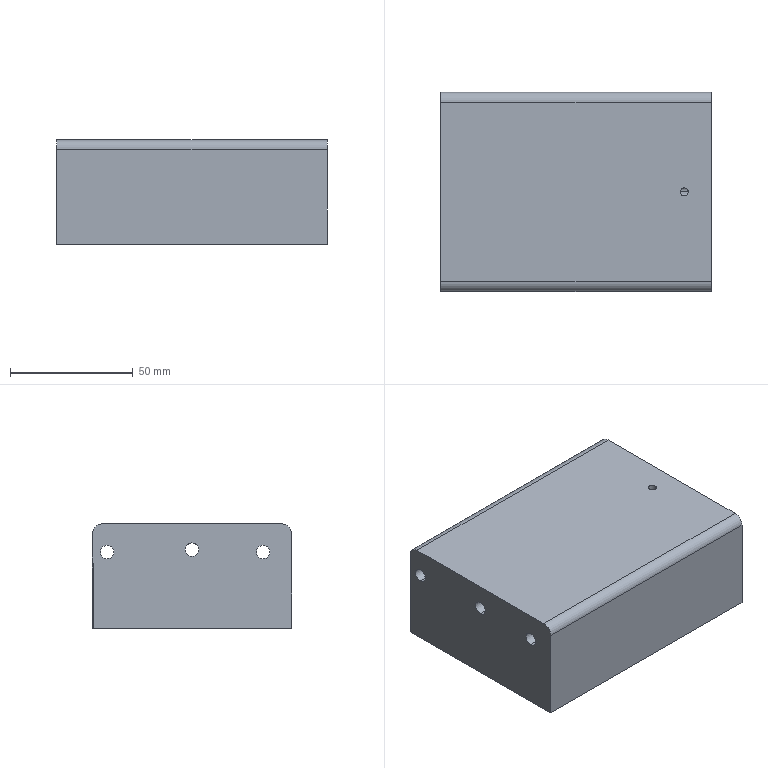Part | STEP file | FFH80-GY-002A^FFH85-B3 -02_three-axis module | 1 solid | 44 faces | box 110 x 81 x 42.5 mm | volume 368601 mm3 | cylinder 25 | plane 13 | cone 6 | commonest cylinder face diameters 5.5 x6 9 x6 4.2 x4 2.5 x2 3 x2 3.3 x2
STEP:
#1=CARTESIAN_POINT('',(102.,18.4,-2.25));
#2=VERTEX_POINT('',#1);
#3=CARTESIAN_POINT('',(102.,22.6,-2.25));
#4=VERTEX_POINT('',#3);
#5=CARTESIAN_POINT('',(102.,20.5,-2.25));
#6=DIRECTION('',(0.,0.,-1.));
#7=DIRECTION('',(0.,1.,0.));
#8=AXIS2_PLACEMENT_3D('',#5,#6,#7);
#9=CIRCLE('',#8,2.1);
#10=EDGE_CURVE('',#2,#4,#9,.T.);
#11=ORIENTED_EDGE('',*,*,#10,.F.);
#12=CARTESIAN_POINT('',(102.,18.4,-21.25));
#13=VERTEX_POINT('',#12);
#14=CARTESIAN_POINT('',(102.,18.4,-21.25));
#15=DIRECTION('',(0.,0.,-1.));
#16=VECTOR('',#15,1000.);
#17=LINE('',#14,#16);
#18=EDGE_CURVE('',#2,#13,#17,.T.);
#19=ORIENTED_EDGE('',*,*,#18,.T.);
#20=CARTESIAN_POINT('',(102.,22.6,-21.25));
#21=VERTEX_POINT('',#20);
#22=CARTESIAN_POINT('',(102.,20.5,-21.25));
#23=DIRECTION('',(0.,0.,-1.));
#24=DIRECTION('',(0.,1.,0.));
#25=AXIS2_PLACEMENT_3D('',#22,#23,#24);
#26=CIRCLE('',#25,2.1);
#27=EDGE_CURVE('',#13,#21,#26,.T.);
#28=ORIENTED_EDGE('',*,*,#27,.T.);
#29=CARTESIAN_POINT('',(102.,22.6,-21.25));
#30=DIRECTION('',(0.,0.,-1.));
#31=VECTOR('',#30,1000.);
#32=LINE('',#29,#31);
#33=EDGE_CURVE('',#4,#21,#32,.T.);
#34=ORIENTED_EDGE('',*,*,#33,.F.);
#35=EDGE_LOOP('',(#11,#19,#28,#34));
#36=FACE_OUTER_BOUND('',#35,.T.);
#37=CARTESIAN_POINT('',(102.,20.5,-21.25));
#38=DIRECTION('',(0.,0.,-1.));
#39=DIRECTION('',(0.,1.,0.));
#40=AXIS2_PLACEMENT_3D('',#37,#38,#39);
#41=CYLINDRICAL_SURFACE('',#40,2.1);
#42=ADVANCED_FACE('',(#36),#41,.F.);
#43=CARTESIAN_POINT('',(102.,-23.6,-2.25));
#44=VERTEX_POINT('',#43);
#45=CARTESIAN_POINT('',(99.9,-21.5,-2.25));
#46=VERTEX_POINT('',#45);
#47=CARTESIAN_POINT('',(102.,-21.5,-2.25));
#48=DIRECTION('',(0.,0.,-1.));
#49=DIRECTION('',(0.,1.,0.));
#50=AXIS2_PLACEMENT_3D('',#47,#48,#49);
#51=CIRCLE('',#50,2.1);
#52=EDGE_CURVE('',#44,#46,#51,.T.);
#53=ORIENTED_EDGE('',*,*,#52,.F.);
#54=CARTESIAN_POINT('',(102.,-23.6,-21.25));
#55=VERTEX_POINT('',#54);
#56=CARTESIAN_POINT('',(102.,-23.6,-21.25));
#57=DIRECTION('',(0.,0.,-1.));
#58=VECTOR('',#57,1000.);
#59=LINE('',#56,#58);
#60=EDGE_CURVE('',#44,#55,#59,.T.);
#61=ORIENTED_EDGE('',*,*,#60,.T.);
#62=CARTESIAN_POINT('',(102.,-19.4,-21.25));
#63=VERTEX_POINT('',#62);
#64=CARTESIAN_POINT('',(102.,-21.5,-21.25));
#65=DIRECTION('',(0.,0.,-1.));
#66=DIRECTION('',(0.,1.,0.));
#67=AXIS2_PLACEMENT_3D('',#64,#65,#66);
#68=CIRCLE('',#67,2.1);
#69=EDGE_CURVE('',#55,#63,#68,.T.);
#70=ORIENTED_EDGE('',*,*,#69,.T.);
#71=CARTESIAN_POINT('',(102.,-19.4,-2.25));
#72=VERTEX_POINT('',#71);
#73=CARTESIAN_POINT('',(102.,-19.4,-21.25));
#74=DIRECTION('',(0.,0.,-1.));
#75=VECTOR('',#74,1000.);
#76=LINE('',#73,#75);
#77=EDGE_CURVE('',#72,#63,#76,.T.);
#78=ORIENTED_EDGE('',*,*,#77,.F.);
#79=CARTESIAN_POINT('',(102.,-21.5,-2.25));
#80=DIRECTION('',(0.,0.,-1.));
#81=DIRECTION('',(0.,1.,0.));
#82=AXIS2_PLACEMENT_3D('',#79,#80,#81);
#83=CIRCLE('',#82,2.1);
#84=EDGE_CURVE('',#46,#72,#83,.T.);
#85=ORIENTED_EDGE('',*,*,#84,.F.);
#86=EDGE_LOOP('',(#53,#61,#70,#78,#85));
#87=FACE_OUTER_BOUND('',#86,.T.);
#88=CARTESIAN_POINT('',(102.,-21.5,-21.25));
#89=DIRECTION('',(0.,0.,-1.));
#90=DIRECTION('',(0.,1.,0.));
#91=AXIS2_PLACEMENT_3D('',#88,#89,#90);
#92=CYLINDRICAL_SURFACE('',#91,2.1);
#93=ADVANCED_FACE('',(#87),#92,.F.);
#94=CARTESIAN_POINT('',(102.,20.5,-0.9882));
#95=VERTEX_POINT('',#94);
#96=CARTESIAN_POINT('',(102.,22.6,-2.25));
#97=DIRECTION('',(0.,0.8572,-0.515));
#98=VECTOR('',#97,1000.);
#99=LINE('',#96,#98);
#100=EDGE_CURVE('',#95,#4,#99,.T.);
#101=ORIENTED_EDGE('',*,*,#100,.F.);
#102=CARTESIAN_POINT('',(102.,18.4,-2.25));
#103=DIRECTION('',(0.,-0.8572,-0.515));
#104=VECTOR('',#103,1000.);
#105=LINE('',#102,#104);
#106=EDGE_CURVE('',#95,#2,#105,.T.);
#107=ORIENTED_EDGE('',*,*,#106,.T.);
#108=ORIENTED_EDGE('',*,*,#10,.T.);
#109=EDGE_LOOP('',(#101,#107,#108));
#110=FACE_OUTER_BOUND('',#109,.T.);
#111=CARTESIAN_POINT('',(102.,20.5,-2.25));
#112=DIRECTION('',(0.,0.,-1.));
#113=DIRECTION('',(0.,1.,0.));
#114=AXIS2_PLACEMENT_3D('',#111,#112,#113);
#115=CONICAL_SURFACE('',#114,2.1,1.03);
#116=ADVANCED_FACE('',(#110),#115,.F.);
#117=CARTESIAN_POINT('',(102.,-21.5,-0.9882));
#118=VERTEX_POINT('',#117);
#119=CARTESIAN_POINT('',(99.9,-21.5,-2.25));
#120=DIRECTION('',(-0.8572,0.,-0.515));
#121=VECTOR('',#120,1000.);
#122=LINE('',#119,#121);
#123=EDGE_CURVE('',#118,#46,#122,.T.);
#124=ORIENTED_EDGE('',*,*,#123,.F.);
#125=CARTESIAN_POINT('',(104.1,-21.5,-2.25));
#126=VERTEX_POINT('',#125);
#127=CARTESIAN_POINT('',(104.1,-21.5,-2.25));
#128=DIRECTION('',(0.8572,0.,-0.515));
#129=VECTOR('',#128,1000.);
#130=LINE('',#127,#129);
#131=EDGE_CURVE('',#118,#126,#130,.T.);
#132=ORIENTED_EDGE('',*,*,#131,.T.);
#133=CARTESIAN_POINT('',(102.,-21.5,-2.25));
#134=DIRECTION('',(0.,0.,-1.));
#135=DIRECTION('',(0.,1.,0.));
#136=AXIS2_PLACEMENT_3D('',#133,#134,#135);
#137=CIRCLE('',#136,2.1);
#138=EDGE_CURVE('',#126,#44,#137,.T.);
#139=ORIENTED_EDGE('',*,*,#138,.T.);
#140=ORIENTED_EDGE('',*,*,#52,.T.);
#141=EDGE_LOOP('',(#124,#132,#139,#140));
#142=FACE_OUTER_BOUND('',#141,.T.);
#143=CARTESIAN_POINT('',(102.,-21.5,-2.25));
#144=DIRECTION('',(0.,0.,-1.));
#145=DIRECTION('',(-1.,0.,0.));
#146=AXIS2_PLACEMENT_3D('',#143,#144,#145);
#147=CONICAL_SURFACE('',#146,2.1,1.03);
#148=ADVANCED_FACE('',(#142),#147,.F.);
#149=CARTESIAN_POINT('',(104.,0.,15.25));
#150=VERTEX_POINT('',#149);
#151=CARTESIAN_POINT('',(104.,0.,6.25));
#152=VERTEX_POINT('',#151);
#153=CARTESIAN_POINT('',(104.,0.,10.75));
#154=DIRECTION('',(1.,0.,0.));
#155=DIRECTION('',(0.,0.,-1.));
#156=AXIS2_PLACEMENT_3D('',#153,#154,#155);
#157=CIRCLE('',#156,4.5);
#158=EDGE_CURVE('',#150,#152,#157,.T.);
#159=ORIENTED_EDGE('',*,*,#158,.F.);
#160=CARTESIAN_POINT('',(110.,0.,15.25));
#161=VERTEX_POINT('',#160);
#162=CARTESIAN_POINT('',(110.,0.,15.25));
#163=DIRECTION('',(1.,0.,0.));
#164=VECTOR('',#163,1000.);
#165=LINE('',#162,#164);
#166=EDGE_CURVE('',#150,#161,#165,.T.);
#167=ORIENTED_EDGE('',*,*,#166,.T.);
#168=CARTESIAN_POINT('',(110.,0.,6.25));
#169=VERTEX_POINT('',#168);
#170=CARTESIAN_POINT('',(110.,0.,10.75));
#171=DIRECTION('',(1.,0.,0.));
#172=DIRECTION('',(0.,0.,-1.));
#173=AXIS2_PLACEMENT_3D('',#170,#171,#172);
#174=CIRCLE('',#173,4.5);
#175=EDGE_CURVE('',#161,#169,#174,.T.);
#176=ORIENTED_EDGE('',*,*,#175,.T.);
#177=CARTESIAN_POINT('',(110.,0.,6.25));
#178=DIRECTION('',(1.,0.,0.));
#179=VECTOR('',#178,1000.);
#180=LINE('',#177,#179);
#181=EDGE_CURVE('',#152,#169,#180,.T.);
#182=ORIENTED_EDGE('',*,*,#181,.F.);
#183=EDGE_LOOP('',(#159,#167,#176,#182));
#184=FACE_OUTER_BOUND('',#183,.T.);
#185=CARTESIAN_POINT('',(110.,0.,10.75));
#186=DIRECTION('',(1.,0.,0.));
#187=DIRECTION('',(0.,0.,-1.));
#188=AXIS2_PLACEMENT_3D('',#185,#186,#187);
#189=CYLINDRICAL_SURFACE('',#188,4.5);
#190=ADVANCED_FACE('',(#184),#189,.F.);
#191=CARTESIAN_POINT('',(104.,34.5,14.25));
#192=VERTEX_POINT('',#191);
#193=CARTESIAN_POINT('',(104.,34.5,5.25));
#194=VERTEX_POINT('',#193);
#195=CARTESIAN_POINT('',(104.,34.5,9.75));
#196=DIRECTION('',(1.,0.,0.));
#197=DIRECTION('',(0.,0.,-1.));
#198=AXIS2_PLACEMENT_3D('',#195,#196,#197);
#199=CIRCLE('',#198,4.5);
#200=EDGE_CURVE('',#192,#194,#199,.T.);
#201=ORIENTED_EDGE('',*,*,#200,.F.);
#202=CARTESIAN_POINT('',(110.,34.5,14.25));
#203=VERTEX_POINT('',#202);
#204=CARTESIAN_POINT('',(110.,34.5,14.25));
#205=DIRECTION('',(1.,0.,0.));
#206=VECTOR('',#205,1000.);
#207=LINE('',#204,#206);
#208=EDGE_CURVE('',#192,#203,#207,.T.);
#209=ORIENTED_EDGE('',*,*,#208,.T.);
#210=CARTESIAN_POINT('',(110.,34.5,5.25));
#211=VERTEX_POINT('',#210);
#212=CARTESIAN_POINT('',(110.,34.5,9.75));
#213=DIRECTION('',(1.,0.,0.));
#214=DIRECTION('',(0.,0.,-1.));
#215=AXIS2_PLACEMENT_3D('',#212,#213,#214);
#216=CIRCLE('',#215,4.5);
#217=EDGE_CURVE('',#203,#211,#216,.T.);
#218=ORIENTED_EDGE('',*,*,#217,.T.);
#219=CARTESIAN_POINT('',(110.,34.5,5.25));
#220=DIRECTION('',(1.,0.,0.));
#221=VECTOR('',#220,1000.);
#222=LINE('',#219,#221);
#223=EDGE_CURVE('',#194,#211,#222,.T.);
#224=ORIENTED_EDGE('',*,*,#223,.F.);
#225=EDGE_LOOP('',(#201,#209,#218,#224));
#226=FACE_OUTER_BOUND('',#225,.T.);
#227=CARTESIAN_POINT('',(110.,34.5,9.75));
#228=DIRECTION('',(1.,0.,0.));
#229=DIRECTION('',(0.,0.,-1.));
#230=AXIS2_PLACEMENT_3D('',#227,#228,#229);
#231=CYLINDRICAL_SURFACE('',#230,4.5);
#232=ADVANCED_FACE('',(#226),#231,.F.);
#233=CARTESIAN_POINT('',(104.,-29.,14.25));
#234=VERTEX_POINT('',#233);
#235=CARTESIAN_POINT('',(104.,-29.,5.25));
#236=VERTEX_POINT('',#235);
#237=CARTESIAN_POINT('',(104.,-29.,9.75));
#238=DIRECTION('',(1.,0.,0.));
#239=DIRECTION('',(0.,0.,-1.));
#240=AXIS2_PLACEMENT_3D('',#237,#238,#239);
#241=CIRCLE('',#240,4.5);
#242=EDGE_CURVE('',#234,#236,#241,.T.);
#243=ORIENTED_EDGE('',*,*,#242,.F.);
#244=CARTESIAN_POINT('',(110.,-29.,14.25));
#245=VERTEX_POINT('',#244);
#246=CARTESIAN_POINT('',(110.,-29.,14.25));
#247=DIRECTION('',(1.,0.,0.));
#248=VECTOR('',#247,1000.);
#249=LINE('',#246,#248);
#250=EDGE_CURVE('',#234,#245,#249,.T.);
#251=ORIENTED_EDGE('',*,*,#250,.T.);
#252=CARTESIAN_POINT('',(110.,-29.,5.25));
#253=VERTEX_POINT('',#252);
#254=CARTESIAN_POINT('',(110.,-29.,9.75));
#255=DIRECTION('',(1.,0.,0.));
#256=DIRECTION('',(0.,0.,-1.));
#257=AXIS2_PLACEMENT_3D('',#254,#255,#256);
#258=CIRCLE('',#257,4.5);
#259=EDGE_CURVE('',#245,#253,#258,.T.);
#260=ORIENTED_EDGE('',*,*,#259,.T.);
#261=CARTESIAN_POINT('',(110.,-29.,5.25));
#262=DIRECTION('',(1.,0.,0.));
#263=VECTOR('',#262,1000.);
#264=LINE('',#261,#263);
#265=EDGE_CURVE('',#236,#253,#264,.T.);
#266=ORIENTED_EDGE('',*,*,#265,.F.);
#267=EDGE_LOOP('',(#243,#251,#260,#266));
#268=FACE_OUTER_BOUND('',#267,.T.);
#269=CARTESIAN_POINT('',(110.,-29.,9.75));
#270=DIRECTION('',(1.,0.,0.));
#271=DIRECTION('',(0.,0.,-1.));
#272=AXIS2_PLACEMENT_3D('',#269,#270,#271);
#273=CYLINDRICAL_SURFACE('',#272,4.5);
#274=ADVANCED_FACE('',(#268),#273,.F.);
#275=CARTESIAN_POINT('',(0.,0.,13.5));
#276=VERTEX_POINT('',#275);
#277=CARTESIAN_POINT('',(0.,0.,8.));
#278=VERTEX_POINT('',#277);
#279=CARTESIAN_POINT('',(0.,0.,10.75));
#280=DIRECTION('',(1.,0.,0.));
#281=DIRECTION('',(0.,0.,-1.));
#282=AXIS2_PLACEMENT_3D('',#279,#280,#281);
#283=CIRCLE('',#282,2.75);
#284=EDGE_CURVE('',#276,#278,#283,.T.);
#285=ORIENTED_EDGE('',*,*,#284,.F.);
#286=CARTESIAN_POINT('',(97.35,0.,13.5));
#287=VERTEX_POINT('',#286);
#288=CARTESIAN_POINT('',(110.,0.,13.5));
#289=DIRECTION('',(1.,0.,0.));
#290=VECTOR('',#289,1000.);
#291=LINE('',#288,#290);
#292=EDGE_CURVE('',#276,#287,#291,.T.);
#293=ORIENTED_EDGE('',*,*,#292,.T.);
#294=CARTESIAN_POINT('',(100.65,0.,13.5));
#295=VERTEX_POINT('',#294);
#296=CARTESIAN_POINT('',(100.65,0.,13.5));
#297=CARTESIAN_POINT('',(100.65,-0.112,13.5));
#298=CARTESIAN_POINT('',(100.639,-0.2216,13.493));
#299=CARTESIAN_POINT('',(100.595,-0.4365,13.467));
#300=CARTESIAN_POINT('',(100.562,-0.5427,13.448));
#301=CARTESIAN_POINT('',(100.436,-0.8412,13.376));
#302=CARTESIAN_POINT('',(100.314,-1.02,13.309));
#303=CARTESIAN_POINT('',(100.091,-1.242,13.205));
#304=CARTESIAN_POINT('',(100.009,-1.31,13.169));
#305=CARTESIAN_POINT('',(99.834,-1.428,13.101));
#306=CARTESIAN_POINT('',(99.741,-1.478,13.07));
#307=CARTESIAN_POINT('',(99.544,-1.561,13.014));
#308=CARTESIAN_POINT('',(99.439,-1.594,12.991));
#309=CARTESIAN_POINT('',(99.224,-1.638,12.959));
#310=CARTESIAN_POINT('',(99.114,-1.65,12.95));
#311=CARTESIAN_POINT('',(98.89,-1.65,12.95));
#312=CARTESIAN_POINT('',(98.781,-1.639,12.958));
#313=CARTESIAN_POINT('',(98.565,-1.595,12.99));
#314=CARTESIAN_POINT('',(98.46,-1.563,13.013));
#315=CARTESIAN_POINT('',(98.262,-1.48,13.068));
#316=CARTESIAN_POINT('',(98.167,-1.428,13.101));
#317=CARTESIAN_POINT('',(97.992,-1.31,13.169));
#318=CARTESIAN_POINT('',(97.911,-1.244,13.204));
#319=CARTESIAN_POINT('',(97.761,-1.095,13.274));
#320=CARTESIAN_POINT('',(97.693,-1.013,13.308));
#321=CARTESIAN_POINT('',(97.575,-0.8379,13.371));
#322=CARTESIAN_POINT('',(97.523,-0.7445,13.399));
#323=CARTESIAN_POINT('',(97.396,-0.444,13.472));
#324=CARTESIAN_POINT('',(97.35,-0.2243,13.5));
#325=CARTESIAN_POINT('',(97.35,0.,13.5));
#326=B_SPLINE_CURVE_WITH_KNOTS('',3,(#296,#297,#298,#299,#300,#301,#302,#303,#304,#305,#306,#307,#308,#309,#310,#311,#312,#313,#314,#315,#316,#317,#318,#319,#320,#321,#322,#323,#324,#325),.UNSPECIFIED.,.F.,.F.,(4,2,2,2,2,2,2,2,2,2,2,2,2,2,4),(0.,0.0003307,0.0006614,0.001323,0.001653,0.001984,0.002315,0.002645,0.002976,0.003307,0.003638,0.003968,0.004299,0.00463,0.005291),.UNSPECIFIED.);
#327=EDGE_CURVE('',#295,#287,#326,.T.);
#328=ORIENTED_EDGE('',*,*,#327,.F.);
#329=CARTESIAN_POINT('',(104.,0.,13.5));
#330=VERTEX_POINT('',#329);
#331=CARTESIAN_POINT('',(110.,0.,13.5));
#332=DIRECTION('',(1.,0.,0.));
#333=VECTOR('',#332,1000.);
#334=LINE('',#331,#333);
#335=EDGE_CURVE('',#295,#330,#334,.T.);
#336=ORIENTED_EDGE('',*,*,#335,.T.);
#337=CARTESIAN_POINT('',(104.,0.,8.));
#338=VERTEX_POINT('',#337);
#339=CARTESIAN_POINT('',(104.,0.,10.75));
#340=DIRECTION('',(-1.,0.,0.));
#341=DIRECTION('',(0.,0.,-1.));
#342=AXIS2_PLACEMENT_3D('',#339,#340,#341);
#343=CIRCLE('',#342,2.75);
#344=EDGE_CURVE('',#338,#330,#343,.T.);
#345=ORIENTED_EDGE('',*,*,#344,.F.);
#346=CARTESIAN_POINT('',(110.,0.,8.));
#347=DIRECTION('',(1.,0.,0.));
#348=VECTOR('',#347,1000.);
#349=LINE('',#346,#348);
#350=EDGE_CURVE('',#278,#338,#349,.T.);
#351=ORIENTED_EDGE('',*,*,#350,.F.);
#352=EDGE_LOOP('',(#285,#293,#328,#336,#345,#351));
#353=FACE_OUTER_BOUND('',#352,.T.);
#354=CARTESIAN_POINT('',(110.,0.,10.75));
#355=DIRECTION('',(1.,0.,0.));
#356=DIRECTION('',(0.,0.,-1.));
#357=AXIS2_PLACEMENT_3D('',#354,#355,#356);
#358=CYLINDRICAL_SURFACE('',#357,2.75);
#359=ADVANCED_FACE('',(#353),#358,.F.);
#360=CARTESIAN_POINT('',(0.,34.5,12.5));
#361=VERTEX_POINT('',#360);
#362=CARTESIAN_POINT('',(0.,34.5,7.));
#363=VERTEX_POINT('',#362);
#364=CARTESIAN_POINT('',(0.,34.5,9.75));
#365=DIRECTION('',(1.,0.,0.));
#366=DIRECTION('',(0.,0.,-1.));
#367=AXIS2_PLACEMENT_3D('',#364,#365,#366);
#368=CIRCLE('',#367,2.75);
#369=EDGE_CURVE('',#361,#363,#368,.T.);
#370=ORIENTED_EDGE('',*,*,#369,.F.);
#371=CARTESIAN_POINT('',(104.,34.5,12.5));
#372=VERTEX_POINT('',#371);
#373=CARTESIAN_POINT('',(110.,34.5,12.5));
#374=DIRECTION('',(1.,0.,0.));
#375=VECTOR('',#374,1000.);
#376=LINE('',#373,#375);
#377=EDGE_CURVE('',#361,#372,#376,.T.);
#378=ORIENTED_EDGE('',*,*,#377,.T.);
#379=CARTESIAN_POINT('',(104.,34.5,7.));
#380=VERTEX_POINT('',#379);
#381=CARTESIAN_POINT('',(104.,34.5,9.75));
#382=DIRECTION('',(-1.,0.,0.));
#383=DIRECTION('',(0.,0.,-1.));
#384=AXIS2_PLACEMENT_3D('',#381,#382,#383);
#385=CIRCLE('',#384,2.75);
#386=EDGE_CURVE('',#380,#372,#385,.T.);
#387=ORIENTED_EDGE('',*,*,#386,.F.);
#388=CARTESIAN_POINT('',(110.,34.5,7.));
#389=DIRECTION('',(1.,0.,0.));
#390=VECTOR('',#389,1000.);
#391=LINE('',#388,#390);
#392=EDGE_CURVE('',#363,#380,#391,.T.);
#393=ORIENTED_EDGE('',*,*,#392,.F.);
#394=EDGE_LOOP('',(#370,#378,#387,#393));
#395=FACE_OUTER_BOUND('',#394,.T.);
#396=CARTESIAN_POINT('',(110.,34.5,9.75));
#397=DIRECTION('',(1.,0.,0.));
#398=DIRECTION('',(0.,0.,-1.));
#399=AXIS2_PLACEMENT_3D('',#396,#397,#398);
#400=CYLINDRICAL_SURFACE('',#399,2.75);
#401=ADVANCED_FACE('',(#395),#400,.F.);
#402=CARTESIAN_POINT('',(0.,-29.,12.5));
#403=VERTEX_POINT('',#402);
#404=CARTESIAN_POINT('',(0.,-29.,7.));
#405=VERTEX_POINT('',#404);
#406=CARTESIAN_POINT('',(0.,-29.,9.75));
#407=DIRECTION('',(1.,0.,0.));
#408=DIRECTION('',(0.,0.,-1.));
#409=AXIS2_PLACEMENT_3D('',#406,#407,#408);
#410=CIRCLE('',#409,2.75);
#411=EDGE_CURVE('',#403,#405,#410,.T.);
#412=ORIENTED_EDGE('',*,*,#411,.F.);
#413=CARTESIAN_POINT('',(104.,-29.,12.5));
#414=VERTEX_POINT('',#413);
#415=CARTESIAN_POINT('',(110.,-29.,12.5));
#416=DIRECTION('',(1.,0.,0.));
#417=VECTOR('',#416,1000.);
#418=LINE('',#415,#417);
#419=EDGE_CURVE('',#403,#414,#418,.T.);
#420=ORIENTED_EDGE('',*,*,#419,.T.);
#421=CARTESIAN_POINT('',(104.,-29.,7.));
#422=VERTEX_POINT('',#421);
#423=CARTESIAN_POINT('',(104.,-29.,9.75));
#424=DIRECTION('',(-1.,0.,0.));
#425=DIRECTION('',(0.,0.,-1.));
#426=AXIS2_PLACEMENT_3D('',#423,#424,#425);
#427=CIRCLE('',#426,2.75);
#428=EDGE_CURVE('',#422,#414,#427,.T.);
#429=ORIENTED_EDGE('',*,*,#428,.F.);
#430=CARTESIAN_POINT('',(110.,-29.,7.));
#431=DIRECTION('',(1.,0.,0.));
#432=VECTOR('',#431,1000.);
#433=LINE('',#430,#432);
#434=EDGE_CURVE('',#405,#422,#433,.T.);
#435=ORIENTED_EDGE('',*,*,#434,.F.);
#436=EDGE_LOOP('',(#412,#420,#429,#435));
#437=FACE_OUTER_BOUND('',#436,.T.);
#438=CARTESIAN_POINT('',(110.,-29.,9.75));
#439=DIRECTION('',(1.,0.,0.));
#440=DIRECTION('',(0.,0.,-1.));
#441=AXIS2_PLACEMENT_3D('',#438,#439,#440);
#442=CYLINDRICAL_SURFACE('',#441,2.75);
#443=ADVANCED_FACE('',(#437),#442,.F.);
#444=CARTESIAN_POINT('',(6.,34.2,-6.75));
#445=VERTEX_POINT('',#444);
#446=CARTESIAN_POINT('',(6.,34.2,-3.75));
#447=VERTEX_POINT('',#446);
#448=CARTESIAN_POINT('',(6.,34.2,-5.25));
#449=DIRECTION('',(0.,1.,0.));
#450=DIRECTION('',(0.,0.,1.));
#451=AXIS2_PLACEMENT_3D('',#448,#449,#450);
#452=CIRCLE('',#451,1.5);
#453=EDGE_CURVE('',#445,#447,#452,.T.);
#454=ORIENTED_EDGE('',*,*,#453,.F.);
#455=CARTESIAN_POINT('',(6.,40.2,-6.75));
#456=VERTEX_POINT('',#455);
#457=CARTESIAN_POINT('',(6.,40.2,-6.75));
#458=DIRECTION('',(0.,1.,0.));
#459=VECTOR('',#458,1000.);
#460=LINE('',#457,#459);
#461=EDGE_CURVE('',#445,#456,#460,.T.);
#462=ORIENTED_EDGE('',*,*,#461,.T.);
#463=CARTESIAN_POINT('',(6.,40.2,-3.75));
#464=VERTEX_POINT('',#463);
#465=CARTESIAN_POINT('',(6.,40.2,-5.25));
#466=DIRECTION('',(0.,-1.,0.));
#467=DIRECTION('',(0.,0.,1.));
#468=AXIS2_PLACEMENT_3D('',#465,#466,#467);
#469=CIRCLE('',#468,1.5);
#470=EDGE_CURVE('',#464,#456,#469,.T.);
#471=ORIENTED_EDGE('',*,*,#470,.F.);
#472=CARTESIAN_POINT('',(6.,40.2,-3.75));
#473=DIRECTION('',(0.,1.,0.));
#474=VECTOR('',#473,1000.);
#475=LINE('',#472,#474);
#476=EDGE_CURVE('',#447,#464,#475,.T.);
#477=ORIENTED_EDGE('',*,*,#476,.F.);
#478=EDGE_LOOP('',(#454,#462,#471,#477));
#479=FACE_OUTER_BOUND('',#478,.T.);
#480=CARTESIAN_POINT('',(6.,40.2,-5.25));
#481=DIRECTION('',(0.,1.,0.));
#482=DIRECTION('',(0.,0.,1.));
#483=AXIS2_PLACEMENT_3D('',#480,#481,#482);
#484=CYLINDRICAL_SURFACE('',#483,1.5);
#485=ADVANCED_FACE('',(#479),#484,.F.);
#486=ORIENTED_EDGE('',*,*,#327,.T.);
#487=CARTESIAN_POINT('',(97.35,0.,21.25));
#488=VERTEX_POINT('',#487);
#489=CARTESIAN_POINT('',(97.35,0.,21.25));
#490=DIRECTION('',(0.,0.,1.));
#491=VECTOR('',#490,1000.);
#492=LINE('',#489,#491);
#493=EDGE_CURVE('',#287,#488,#492,.T.);
#494=ORIENTED_EDGE('',*,*,#493,.T.);
#495=CARTESIAN_POINT('',(100.65,0.,21.25));
#496=VERTEX_POINT('',#495);
#497=CARTESIAN_POINT('',(99.,0.,21.25));
#498=DIRECTION('',(0.,0.,1.));
#499=DIRECTION('',(1.,0.,0.));
#500=AXIS2_PLACEMENT_3D('',#497,#498,#499);
#501=CIRCLE('',#500,1.65);
#502=EDGE_CURVE('',#488,#496,#501,.T.);
#503=ORIENTED_EDGE('',*,*,#502,.T.);
#504=CARTESIAN_POINT('',(100.65,0.,21.25));
#505=DIRECTION('',(0.,0.,1.));
#506=VECTOR('',#505,1000.);
#507=LINE('',#504,#506);
#508=EDGE_CURVE('',#295,#496,#507,.T.);
#509=ORIENTED_EDGE('',*,*,#508,.F.);
#510=EDGE_LOOP('',(#486,#494,#503,#509));
#511=FACE_OUTER_BOUND('',#510,.T.);
#512=CARTESIAN_POINT('',(99.,0.,21.25));
#513=DIRECTION('',(0.,0.,1.));
#514=DIRECTION('',(1.,0.,0.));
#515=AXIS2_PLACEMENT_3D('',#512,#513,#514);
#516=CYLINDRICAL_SURFACE('',#515,1.65);
#517=ADVANCED_FACE('',(#511),#516,.F.);
#518=CARTESIAN_POINT('',(6.,31.7,-6.5));
#519=VERTEX_POINT('',#518);
#520=CARTESIAN_POINT('',(6.,31.7,-4.));
#521=VERTEX_POINT('',#520);
#522=CARTESIAN_POINT('',(6.,31.7,-5.25));
#523=DIRECTION('',(0.,1.,0.));
#524=DIRECTION('',(0.,0.,1.));
#525=AXIS2_PLACEMENT_3D('',#522,#523,#524);
#526=CIRCLE('',#525,1.25);
#527=EDGE_CURVE('',#519,#521,#526,.T.);
#528=ORIENTED_EDGE('',*,*,#527,.F.);
#529=CARTESIAN_POINT('',(6.,34.2,-6.5));
#530=VERTEX_POINT('',#529);
#531=CARTESIAN_POINT('',(6.,40.2,-6.5));
#532=DIRECTION('',(0.,1.,0.));
#533=VECTOR('',#532,1000.);
#534=LINE('',#531,#533);
#535=EDGE_CURVE('',#519,#530,#534,.T.);
#536=ORIENTED_EDGE('',*,*,#535,.T.);
#537=CARTESIAN_POINT('',(6.,34.2,-4.));
#538=VERTEX_POINT('',#537);
#539=CARTESIAN_POINT('',(6.,34.2,-5.25));
#540=DIRECTION('',(0.,1.,0.));
#541=DIRECTION('',(0.,0.,1.));
#542=AXIS2_PLACEMENT_3D('',#539,#540,#541);
#543=CIRCLE('',#542,1.25);
#544=EDGE_CURVE('',#530,#538,#543,.T.);
#545=ORIENTED_EDGE('',*,*,#544,.T.);
#546=CARTESIAN_POINT('',(6.,40.2,-4.));
#547=DIRECTION('',(0.,1.,0.));
#548=VECTOR('',#547,1000.);
#549=LINE('',#546,#548);
#550=EDGE_CURVE('',#521,#538,#549,.T.);
#551=ORIENTED_EDGE('',*,*,#550,.F.);
#552=EDGE_LOOP('',(#528,#536,#545,#551));
#553=FACE_OUTER_BOUND('',#552,.T.);
#554=CARTESIAN_POINT('',(6.,40.2,-5.25));
#555=DIRECTION('',(0.,1.,0.));
#556=DIRECTION('',(0.,0.,1.));
#557=AXIS2_PLACEMENT_3D('',#554,#555,#556);
#558=CYLINDRICAL_SURFACE('',#557,1.25);
#559=ADVANCED_FACE('',(#553),#558,.F.);
#560=CARTESIAN_POINT('',(6.,30.949,-5.25));
#561=VERTEX_POINT('',#560);
#562=CARTESIAN_POINT('',(6.,31.7,-4.));
#563=DIRECTION('',(0.,0.515,0.8572));
#564=VECTOR('',#563,1000.);
#565=LINE('',#562,#564);
#566=EDGE_CURVE('',#561,#521,#565,.T.);
#567=ORIENTED_EDGE('',*,*,#566,.F.);
#568=CARTESIAN_POINT('',(6.,31.7,-6.5));
#569=DIRECTION('',(0.,0.515,-0.8572));
#570=VECTOR('',#569,1000.);
#571=LINE('',#568,#570);
#572=EDGE_CURVE('',#561,#519,#571,.T.);
#573=ORIENTED_EDGE('',*,*,#572,.T.);
#574=ORIENTED_EDGE('',*,*,#527,.T.);
#575=EDGE_LOOP('',(#567,#573,#574));
#576=FACE_OUTER_BOUND('',#575,.T.);
#577=CARTESIAN_POINT('',(6.,31.7,-5.25));
#578=DIRECTION('',(0.,1.,0.));
#579=DIRECTION('',(0.,0.,1.));
#580=AXIS2_PLACEMENT_3D('',#577,#578,#579);
#581=CONICAL_SURFACE('',#580,1.25,1.03);
#582=ADVANCED_FACE('',(#576),#581,.F.);
#583=CARTESIAN_POINT('',(102.,20.5,-21.25));
#584=DIRECTION('',(0.,0.,-1.));
#585=DIRECTION('',(0.,1.,0.));
#586=AXIS2_PLACEMENT_3D('',#583,#584,#585);
#587=CIRCLE('',#586,2.1);
#588=EDGE_CURVE('',#21,#13,#587,.T.);
#589=ORIENTED_EDGE('',*,*,#588,.F.);
#590=ORIENTED_EDGE('',*,*,#27,.F.);
#591=EDGE_LOOP('',(#589,#590));
#592=FACE_BOUND('',#591,.T.);
#593=CARTESIAN_POINT('',(102.,-21.5,-21.25));
#594=DIRECTION('',(0.,0.,-1.));
#595=DIRECTION('',(0.,1.,0.));
#596=AXIS2_PLACEMENT_3D('',#593,#594,#595);
#597=CIRCLE('',#596,2.1);
#598=EDGE_CURVE('',#63,#55,#597,.T.);
#599=ORIENTED_EDGE('',*,*,#598,.F.);
#600=ORIENTED_EDGE('',*,*,#69,.F.);
#601=EDGE_LOOP('',(#599,#600));
#602=FACE_BOUND('',#601,.T.);
#603=CARTESIAN_POINT('',(110.,40.5,-21.25));
#604=VERTEX_POINT('',#603);
#605=CARTESIAN_POINT('',(12.5,40.5,-21.25));
#606=VERTEX_POINT('',#605);
#607=CARTESIAN_POINT('',(110.,40.5,-21.25));
#608=DIRECTION('',(-1.,0.,0.));
#609=VECTOR('',#608,1000.);
#610=LINE('',#607,#609);
#611=EDGE_CURVE('',#604,#606,#610,.T.);
#612=ORIENTED_EDGE('',*,*,#611,.F.);
#613=CARTESIAN_POINT('',(110.,-40.5,-21.25));
#614=VERTEX_POINT('',#613);
#615=CARTESIAN_POINT('',(110.,40.5,-21.25));
#616=DIRECTION('',(0.,1.,0.));
#617=VECTOR('',#616,1000.);
#618=LINE('',#615,#617);
#619=EDGE_CURVE('',#614,#604,#618,.T.);
#620=ORIENTED_EDGE('',*,*,#619,.F.);
#621=CARTESIAN_POINT('',(0.,-40.5,-21.25));
#622=VERTEX_POINT('',#621);
#623=CARTESIAN_POINT('',(110.,-40.5,-21.25));
#624=DIRECTION('',(1.,0.,0.));
#625=VECTOR('',#624,1000.);
#626=LINE('',#623,#625);
#627=EDGE_CURVE('',#622,#614,#626,.T.);
#628=ORIENTED_EDGE('',*,*,#627,.F.);
#629=CARTESIAN_POINT('',(0.,40.2,-21.25));
#630=VERTEX_POINT('',#629);
#631=CARTESIAN_POINT('',(0.,40.5,-21.25));
#632=DIRECTION('',(0.,-1.,0.));
#633=VECTOR('',#632,1000.);
#634=LINE('',#631,#633);
#635=EDGE_CURVE('',#630,#622,#634,.T.);
#636=ORIENTED_EDGE('',*,*,#635,.F.);
#637=CARTESIAN_POINT('',(12.5,40.2,-21.25));
#638=VERTEX_POINT('',#637);
#639=CARTESIAN_POINT('',(110.,40.2,-21.25));
#640=DIRECTION('',(-1.,0.,0.));
#641=VECTOR('',#640,1000.);
#642=LINE('',#639,#641);
#643=EDGE_CURVE('',#638,#630,#642,.T.);
#644=ORIENTED_EDGE('',*,*,#643,.F.);
#645=CARTESIAN_POINT('',(12.5,40.2,-21.25));
#646=DIRECTION('',(0.,1.,0.));
#647=VECTOR('',#646,1000.);
#648=LINE('',#645,#647);
#649=EDGE_CURVE('',#638,#606,#648,.T.);
#650=ORIENTED_EDGE('',*,*,#649,.T.);
#651=EDGE_LOOP('',(#612,#620,#628,#636,#644,#650));
#652=FACE_OUTER_BOUND('',#651,.T.);
#653=CARTESIAN_POINT('',(110.,40.5,-21.25));
#654=DIRECTION('',(0.,0.,1.));
#655=DIRECTION('',(0.,-1.,0.));
#656=AXIS2_PLACEMENT_3D('',#653,#654,#655);
#657=PLANE('',#656);
#658=ADVANCED_FACE('',(#592,#602,#652),#657,.F.);
#659=ORIENTED_EDGE('',*,*,#18,.F.);
#660=CARTESIAN_POINT('',(102.,20.5,-2.25));
#661=DIRECTION('',(0.,0.,-1.));
#662=DIRECTION('',(0.,1.,0.));
#663=AXIS2_PLACEMENT_3D('',#660,#661,#662);
#664=CIRCLE('',#663,2.1);
#665=EDGE_CURVE('',#4,#2,#664,.T.);
#666=ORIENTED_EDGE('',*,*,#665,.F.);
#667=ORIENTED_EDGE('',*,*,#33,.T.);
#668=ORIENTED_EDGE('',*,*,#588,.T.);
#669=EDGE_LOOP('',(#659,#666,#667,#668));
#670=FACE_OUTER_BOUND('',#669,.T.);
#671=CARTESIAN_POINT('',(102.,20.5,-21.25));
#672=DIRECTION('',(0.,0.,-1.));
#673=DIRECTION('',(0.,1.,0.));
#674=AXIS2_PLACEMENT_3D('',#671,#672,#673);
#675=CYLINDRICAL_SURFACE('',#674,2.1);
#676=ADVANCED_FACE('',(#670),#675,.F.);
#677=ORIENTED_EDGE('',*,*,#60,.F.);
#678=ORIENTED_EDGE('',*,*,#138,.F.);
#679=CARTESIAN_POINT('',(102.,-21.5,-2.25));
#680=DIRECTION('',(0.,0.,-1.));
#681=DIRECTION('',(0.,1.,0.));
#682=AXIS2_PLACEMENT_3D('',#679,#680,#681);
#683=CIRCLE('',#682,2.1);
#684=EDGE_CURVE('',#72,#126,#683,.T.);
#685=ORIENTED_EDGE('',*,*,#684,.F.);
#686=ORIENTED_EDGE('',*,*,#77,.T.);
#687=ORIENTED_EDGE('',*,*,#598,.T.);
#688=EDGE_LOOP('',(#677,#678,#685,#686,#687));
#689=FACE_OUTER_BOUND('',#688,.T.);
#690=CARTESIAN_POINT('',(102.,-21.5,-21.25));
#691=DIRECTION('',(0.,0.,-1.));
#692=DIRECTION('',(0.,1.,0.));
#693=AXIS2_PLACEMENT_3D('',#690,#691,#692);
#694=CYLINDRICAL_SURFACE('',#693,2.1);
#695=ADVANCED_FACE('',(#689),#694,.F.);
#696=CARTESIAN_POINT('',(10.5,40.5,5.25));
#697=VERTEX_POINT('',#696);
#698=CARTESIAN_POINT('',(12.5,40.5,3.25));
#699=VERTEX_POINT('',#698);
#700=CARTESIAN_POINT('',(10.5,40.5,3.25));
#701=DIRECTION('',(0.,1.,0.));
#702=DIRECTION('',(0.,0.,-1.));
#703=AXIS2_PLACEMENT_3D('',#700,#701,#702);
#704=CIRCLE('',#703,2.);
#705=EDGE_CURVE('',#697,#699,#704,.T.);
#706=ORIENTED_EDGE('',*,*,#705,.F.);
#707=CARTESIAN_POINT('',(0.,40.5,5.25));
#708=VERTEX_POINT('',#707);
#709=CARTESIAN_POINT('',(110.,40.5,5.25));
#710=DIRECTION('',(1.,0.,0.));
#711=VECTOR('',#710,1000.);
#712=LINE('',#709,#711);
#713=EDGE_CURVE('',#708,#697,#712,.T.);
#714=ORIENTED_EDGE('',*,*,#713,.F.);
#715=CARTESIAN_POINT('',(0.,40.5,17.25));
#716=VERTEX_POINT('',#715);
#717=CARTESIAN_POINT('',(0.,40.5,-21.25));
#718=DIRECTION('',(0.,0.,-1.));
#719=VECTOR('',#718,1000.);
#720=LINE('',#717,#719);
#721=EDGE_CURVE('',#716,#708,#720,.T.);
#722=ORIENTED_EDGE('',*,*,#721,.F.);
#723=CARTESIAN_POINT('',(110.,40.5,17.25));
#724=VERTEX_POINT('',#723);
#725=CARTESIAN_POINT('',(110.,40.5,17.25));
#726=DIRECTION('',(-1.,0.,0.));
#727=VECTOR('',#726,1000.);
#728=LINE('',#725,#727);
#729=EDGE_CURVE('',#724,#716,#728,.T.);
#730=ORIENTED_EDGE('',*,*,#729,.F.);
#731=CARTESIAN_POINT('',(110.,40.5,-21.25));
#732=DIRECTION('',(0.,0.,1.));
#733=VECTOR('',#732,1000.);
#734=LINE('',#731,#733);
#735=EDGE_CURVE('',#604,#724,#734,.T.);
#736=ORIENTED_EDGE('',*,*,#735,.F.);
#737=ORIENTED_EDGE('',*,*,#611,.T.);
#738=CARTESIAN_POINT('',(12.5,40.5,-21.25));
#739=DIRECTION('',(0.,0.,-1.));
#740=VECTOR('',#739,1000.);
#741=LINE('',#738,#740);
#742=EDGE_CURVE('',#699,#606,#741,.T.);
#743=ORIENTED_EDGE('',*,*,#742,.F.);
#744=EDGE_LOOP('',(#706,#714,#722,#730,#736,#737,#743));
#745=FACE_OUTER_BOUND('',#744,.T.);
#746=CARTESIAN_POINT('',(110.,40.5,-21.25));
#747=DIRECTION('',(0.,-1.,0.));
#748=DIRECTION('',(0.,0.,-1.));
#749=AXIS2_PLACEMENT_3D('',#746,#747,#748);
#750=PLANE('',#749);
#751=ADVANCED_FACE('',(#745),#750,.F.);
#752=CARTESIAN_POINT('',(110.,0.,10.75));
#753=DIRECTION('',(1.,0.,0.));
#754=DIRECTION('',(0.,0.,-1.));
#755=AXIS2_PLACEMENT_3D('',#752,#753,#754);
#756=CIRCLE('',#755,4.5);
#757=EDGE_CURVE('',#169,#161,#756,.T.);
#758=ORIENTED_EDGE('',*,*,#757,.F.);
#759=ORIENTED_EDGE('',*,*,#175,.F.);
#760=EDGE_LOOP('',(#758,#759));
#761=FACE_BOUND('',#760,.T.);
#762=CARTESIAN_POINT('',(110.,34.5,9.75));
#763=DIRECTION('',(1.,0.,0.));
#764=DIRECTION('',(0.,0.,-1.));
#765=AXIS2_PLACEMENT_3D('',#762,#763,#764);
#766=CIRCLE('',#765,4.5);
#767=EDGE_CURVE('',#211,#203,#766,.T.);
#768=ORIENTED_EDGE('',*,*,#767,.F.);
#769=ORIENTED_EDGE('',*,*,#217,.F.);
#770=EDGE_LOOP('',(#768,#769));
#771=FACE_BOUND('',#770,.T.);
#772=CARTESIAN_POINT('',(110.,-29.,9.75));
#773=DIRECTION('',(1.,0.,0.));
#774=DIRECTION('',(0.,0.,-1.));
#775=AXIS2_PLACEMENT_3D('',#772,#773,#774);
#776=CIRCLE('',#775,4.5);
#777=EDGE_CURVE('',#253,#245,#776,.T.);
#778=ORIENTED_EDGE('',*,*,#777,.F.);
#779=ORIENTED_EDGE('',*,*,#259,.F.);
#780=EDGE_LOOP('',(#778,#779));
#781=FACE_BOUND('',#780,.T.);
#782=CARTESIAN_POINT('',(110.,-40.5,17.25));
#783=VERTEX_POINT('',#782);
#784=CARTESIAN_POINT('',(110.,-40.5,0.));
#785=DIRECTION('',(0.,0.,1.));
#786=VECTOR('',#785,1000.);
#787=LINE('',#784,#786);
#788=EDGE_CURVE('',#614,#783,#787,.T.);
#789=ORIENTED_EDGE('',*,*,#788,.F.);
#790=ORIENTED_EDGE('',*,*,#619,.T.);
#791=ORIENTED_EDGE('',*,*,#735,.T.);
#792=CARTESIAN_POINT('',(110.,36.5,21.25));
#793=VERTEX_POINT('',#792);
#794=CARTESIAN_POINT('',(110.,36.5,17.25));
#795=DIRECTION('',(-1.,0.,0.));
#796=DIRECTION('',(0.,0.,1.));
#797=AXIS2_PLACEMENT_3D('',#794,#795,#796);
#798=CIRCLE('',#797,4.);
#799=EDGE_CURVE('',#793,#724,#798,.T.);
#800=ORIENTED_EDGE('',*,*,#799,.F.);
#801=CARTESIAN_POINT('',(110.,-36.5,21.25));
#802=VERTEX_POINT('',#801);
#803=CARTESIAN_POINT('',(110.,0.,21.25));
#804=DIRECTION('',(0.,1.,0.));
#805=VECTOR('',#804,1000.);
#806=LINE('',#803,#805);
#807=EDGE_CURVE('',#802,#793,#806,.T.);
#808=ORIENTED_EDGE('',*,*,#807,.F.);
#809=CARTESIAN_POINT('',(110.,-36.5,17.25));
#810=DIRECTION('',(-1.,0.,0.));
#811=DIRECTION('',(0.,0.,1.));
#812=AXIS2_PLACEMENT_3D('',#809,#810,#811);
#813=CIRCLE('',#812,4.);
#814=EDGE_CURVE('',#783,#802,#813,.T.);
#815=ORIENTED_EDGE('',*,*,#814,.F.);
#816=EDGE_LOOP('',(#789,#790,#791,#800,#808,#815));
#817=FACE_OUTER_BOUND('',#816,.T.);
#818=CARTESIAN_POINT('',(110.,0.,0.));
#819=DIRECTION('',(-1.,0.,0.));
#820=DIRECTION('',(0.,0.,1.));
#821=AXIS2_PLACEMENT_3D('',#818,#819,#820);
#822=PLANE('',#821);
#823=ADVANCED_FACE('',(#761,#771,#781,#817),#822,.F.);
#824=CARTESIAN_POINT('',(0.,-40.5,17.25));
#825=VERTEX_POINT('',#824);
#826=CARTESIAN_POINT('',(0.,-40.5,-21.25));
#827=DIRECTION('',(0.,0.,1.));
#828=VECTOR('',#827,1000.);
#829=LINE('',#826,#828);
#830=EDGE_CURVE('',#622,#825,#829,.T.);
#831=ORIENTED_EDGE('',*,*,#830,.F.);
#832=ORIENTED_EDGE('',*,*,#627,.T.);
#833=ORIENTED_EDGE('',*,*,#788,.T.);
#834=CARTESIAN_POINT('',(110.,-40.5,17.25));
#835=DIRECTION('',(1.,0.,0.));
#836=VECTOR('',#835,1000.);
#837=LINE('',#834,#836);
#838=EDGE_CURVE('',#825,#783,#837,.T.);
#839=ORIENTED_EDGE('',*,*,#838,.F.);
#840=EDGE_LOOP('',(#831,#832,#833,#839));
#841=FACE_OUTER_BOUND('',#840,.T.);
#842=CARTESIAN_POINT('',(110.,-40.5,-21.25));
#843=DIRECTION('',(0.,1.,0.));
#844=DIRECTION('',(0.,0.,1.));
#845=AXIS2_PLACEMENT_3D('',#842,#843,#844);
#846=PLANE('',#845);
#847=ADVANCED_FACE('',(#841),#846,.F.);
#848=CARTESIAN_POINT('',(0.,-36.5,21.25));
#849=VERTEX_POINT('',#848);
#850=CARTESIAN_POINT('',(0.,-36.5,17.25));
#851=DIRECTION('',(-1.,0.,0.));
#852=DIRECTION('',(0.,0.,1.));
#853=AXIS2_PLACEMENT_3D('',#850,#851,#852);
#854=CIRCLE('',#853,4.);
#855=EDGE_CURVE('',#825,#849,#854,.T.);
#856=ORIENTED_EDGE('',*,*,#855,.T.);
#857=CARTESIAN_POINT('',(0.,36.5,21.25));
#858=VERTEX_POINT('',#857);
#859=CARTESIAN_POINT('',(0.,0.,21.25));
#860=DIRECTION('',(0.,1.,0.));
#861=VECTOR('',#860,1000.);
#862=LINE('',#859,#861);
#863=EDGE_CURVE('',#849,#858,#862,.T.);
#864=ORIENTED_EDGE('',*,*,#863,.T.);
#865=CARTESIAN_POINT('',(0.,36.5,17.25));
#866=DIRECTION('',(-1.,0.,0.));
#867=DIRECTION('',(0.,0.,1.));
#868=AXIS2_PLACEMENT_3D('',#865,#866,#867);
#869=CIRCLE('',#868,4.);
#870=EDGE_CURVE('',#858,#716,#869,.T.);
#871=ORIENTED_EDGE('',*,*,#870,.T.);
#872=ORIENTED_EDGE('',*,*,#721,.T.);
#873=CARTESIAN_POINT('',(0.,40.2,5.25));
#874=VERTEX_POINT('',#873);
#875=CARTESIAN_POINT('',(0.,0.,5.25));
#876=DIRECTION('',(0.,-1.,0.));
#877=VECTOR('',#876,1000.);
#878=LINE('',#875,#877);
#879=EDGE_CURVE('',#708,#874,#878,.T.);
#880=ORIENTED_EDGE('',*,*,#879,.T.);
#881=CARTESIAN_POINT('',(0.,40.2,0.));
#882=DIRECTION('',(0.,0.,-1.));
#883=VECTOR('',#882,1000.);
#884=LINE('',#881,#883);
#885=EDGE_CURVE('',#874,#630,#884,.T.);
#886=ORIENTED_EDGE('',*,*,#885,.T.);
#887=ORIENTED_EDGE('',*,*,#635,.T.);
#888=ORIENTED_EDGE('',*,*,#830,.T.);
#889=EDGE_LOOP('',(#856,#864,#871,#872,#880,#886,#887,#888));
#890=FACE_OUTER_BOUND('',#889,.T.);
#891=CARTESIAN_POINT('',(0.,0.,10.75));
#892=DIRECTION('',(1.,0.,0.));
#893=DIRECTION('',(0.,0.,-1.));
#894=AXIS2_PLACEMENT_3D('',#891,#892,#893);
#895=CIRCLE('',#894,2.75);
#896=EDGE_CURVE('',#278,#276,#895,.T.);
#897=ORIENTED_EDGE('',*,*,#896,.T.);
#898=ORIENTED_EDGE('',*,*,#284,.T.);
#899=EDGE_LOOP('',(#897,#898));
#900=FACE_BOUND('',#899,.T.);
#901=CARTESIAN_POINT('',(0.,34.5,9.75));
#902=DIRECTION('',(1.,0.,0.));
#903=DIRECTION('',(0.,0.,-1.));
#904=AXIS2_PLACEMENT_3D('',#901,#902,#903);
#905=CIRCLE('',#904,2.75);
#906=EDGE_CURVE('',#363,#361,#905,.T.);
#907=ORIENTED_EDGE('',*,*,#906,.T.);
#908=ORIENTED_EDGE('',*,*,#369,.T.);
#909=EDGE_LOOP('',(#907,#908));
#910=FACE_BOUND('',#909,.T.);
#911=CARTESIAN_POINT('',(0.,-29.,9.75));
#912=DIRECTION('',(1.,0.,0.));
#913=DIRECTION('',(0.,0.,-1.));
#914=AXIS2_PLACEMENT_3D('',#911,#912,#913);
#915=CIRCLE('',#914,2.75);
#916=EDGE_CURVE('',#405,#403,#915,.T.);
#917=ORIENTED_EDGE('',*,*,#916,.T.);
#918=ORIENTED_EDGE('',*,*,#411,.T.);
#919=EDGE_LOOP('',(#917,#918));
#920=FACE_BOUND('',#919,.T.);
#921=CARTESIAN_POINT('',(0.,0.,0.));
#922=DIRECTION('',(-1.,0.,0.));
#923=DIRECTION('',(0.,0.,1.));
#924=AXIS2_PLACEMENT_3D('',#921,#922,#923);
#925=PLANE('',#924);
#926=ADVANCED_FACE('',(#890,#900,#910,#920),#925,.T.);
#927=ORIENTED_EDGE('',*,*,#470,.T.);
#928=CARTESIAN_POINT('',(6.,40.2,-5.25));
#929=DIRECTION('',(0.,-1.,0.));
#930=DIRECTION('',(0.,0.,1.));
#931=AXIS2_PLACEMENT_3D('',#928,#929,#930);
#932=CIRCLE('',#931,1.5);
#933=EDGE_CURVE('',#456,#464,#932,.T.);
#934=ORIENTED_EDGE('',*,*,#933,.T.);
#935=EDGE_LOOP('',(#927,#934));
#936=FACE_BOUND('',#935,.T.);
#937=CARTESIAN_POINT('',(10.5,40.2,5.25));
#938=VERTEX_POINT('',#937);
#939=CARTESIAN_POINT('',(12.5,40.2,3.25));
#940=VERTEX_POINT('',#939);
#941=CARTESIAN_POINT('',(10.5,40.2,3.25));
#942=DIRECTION('',(0.,1.,0.));
#943=DIRECTION('',(0.,0.,-1.));
#944=AXIS2_PLACEMENT_3D('',#941,#942,#943);
#945=CIRCLE('',#944,2.);
#946=EDGE_CURVE('',#938,#940,#945,.T.);
#947=ORIENTED_EDGE('',*,*,#946,.T.);
#948=CARTESIAN_POINT('',(12.5,40.2,0.));
#949=DIRECTION('',(0.,0.,-1.));
#950=VECTOR('',#949,1000.);
#951=LINE('',#948,#950);
#952=EDGE_CURVE('',#940,#638,#951,.T.);
#953=ORIENTED_EDGE('',*,*,#952,.T.);
#954=ORIENTED_EDGE('',*,*,#643,.T.);
#955=ORIENTED_EDGE('',*,*,#885,.F.);
#956=CARTESIAN_POINT('',(0.,40.2,5.25));
#957=DIRECTION('',(1.,0.,0.));
#958=VECTOR('',#957,1000.);
#959=LINE('',#956,#958);
#960=EDGE_CURVE('',#874,#938,#959,.T.);
#961=ORIENTED_EDGE('',*,*,#960,.T.);
#962=EDGE_LOOP('',(#947,#953,#954,#955,#961));
#963=FACE_OUTER_BOUND('',#962,.T.);
#964=CARTESIAN_POINT('',(0.,40.2,0.));
#965=DIRECTION('',(0.,1.,0.));
#966=DIRECTION('',(0.,0.,1.));
#967=AXIS2_PLACEMENT_3D('',#964,#965,#966);
#968=PLANE('',#967);
#969=ADVANCED_FACE('',(#936,#963),#968,.T.);
#970=ORIENTED_EDGE('',*,*,#106,.F.);
#971=ORIENTED_EDGE('',*,*,#100,.T.);
#972=ORIENTED_EDGE('',*,*,#665,.T.);
#973=EDGE_LOOP('',(#970,#971,#972));
#974=FACE_OUTER_BOUND('',#973,.T.);
#975=CARTESIAN_POINT('',(102.,20.5,-2.25));
#976=DIRECTION('',(0.,0.,-1.));
#977=DIRECTION('',(0.,1.,0.));
#978=AXIS2_PLACEMENT_3D('',#975,#976,#977);
#979=CONICAL_SURFACE('',#978,2.1,1.03);
#980=ADVANCED_FACE('',(#974),#979,.F.);
#981=ORIENTED_EDGE('',*,*,#131,.F.);
#982=ORIENTED_EDGE('',*,*,#123,.T.);
#983=ORIENTED_EDGE('',*,*,#84,.T.);
#984=ORIENTED_EDGE('',*,*,#684,.T.);
#985=EDGE_LOOP('',(#981,#982,#983,#984));
#986=FACE_OUTER_BOUND('',#985,.T.);
#987=CARTESIAN_POINT('',(102.,-21.5,-2.25));
#988=DIRECTION('',(0.,0.,-1.));
#989=DIRECTION('',(-1.,0.,0.));
#990=AXIS2_PLACEMENT_3D('',#987,#988,#989);
#991=CONICAL_SURFACE('',#990,2.1,1.03);
#992=ADVANCED_FACE('',(#986),#991,.F.);
#993=ORIENTED_EDGE('',*,*,#742,.T.);
#994=ORIENTED_EDGE('',*,*,#649,.F.);
#995=ORIENTED_EDGE('',*,*,#952,.F.);
#996=CARTESIAN_POINT('',(12.5,40.2,3.25));
#997=DIRECTION('',(0.,-1.,0.));
#998=VECTOR('',#997,1000.);
#999=LINE('',#996,#998);
#1000=EDGE_CURVE('',#699,#940,#999,.T.);
#1001=ORIENTED_EDGE('',*,*,#1000,.F.);
#1002=EDGE_LOOP('',(#993,#994,#995,#1001));
#1003=FACE_OUTER_BOUND('',#1002,.T.);
#1004=CARTESIAN_POINT('',(12.5,40.2,5.25));
#1005=DIRECTION('',(1.,0.,0.));
#1006=DIRECTION('',(0.,0.,-1.));
#1007=AXIS2_PLACEMENT_3D('',#1004,#1005,#1006);
#1008=PLANE('',#1007);
#1009=ADVANCED_FACE('',(#1003),#1008,.F.);
#1010=ORIENTED_EDGE('',*,*,#705,.T.);
#1011=ORIENTED_EDGE('',*,*,#1000,.T.);
#1012=ORIENTED_EDGE('',*,*,#946,.F.);
#1013=CARTESIAN_POINT('',(10.5,40.2,5.25));
#1014=DIRECTION('',(0.,-1.,0.));
#1015=VECTOR('',#1014,1000.);
#1016=LINE('',#1013,#1015);
#1017=EDGE_CURVE('',#697,#938,#1016,.T.);
#1018=ORIENTED_EDGE('',*,*,#1017,.F.);
#1019=EDGE_LOOP('',(#1010,#1011,#1012,#1018));
#1020=FACE_OUTER_BOUND('',#1019,.T.);
#1021=CARTESIAN_POINT('',(10.5,40.2,3.25));
#1022=DIRECTION('',(0.,-1.,0.));
#1023=DIRECTION('',(0.,0.,-1.));
#1024=AXIS2_PLACEMENT_3D('',#1021,#1022,#1023);
#1025=CYLINDRICAL_SURFACE('',#1024,2.);
#1026=ADVANCED_FACE('',(#1020),#1025,.F.);
#1027=ORIENTED_EDGE('',*,*,#960,.F.);
#1028=ORIENTED_EDGE('',*,*,#879,.F.);
#1029=ORIENTED_EDGE('',*,*,#713,.T.);
#1030=ORIENTED_EDGE('',*,*,#1017,.T.);
#1031=EDGE_LOOP('',(#1027,#1028,#1029,#1030));
#1032=FACE_OUTER_BOUND('',#1031,.T.);
#1033=CARTESIAN_POINT('',(12.5,40.2,5.25));
#1034=DIRECTION('',(0.,0.,1.));
#1035=DIRECTION('',(0.,-1.,0.));
#1036=AXIS2_PLACEMENT_3D('',#1033,#1034,#1035);
#1037=PLANE('',#1036);
#1038=ADVANCED_FACE('',(#1032),#1037,.F.);
#1039=ORIENTED_EDGE('',*,*,#799,.T.);
#1040=ORIENTED_EDGE('',*,*,#729,.T.);
#1041=ORIENTED_EDGE('',*,*,#870,.F.);
#1042=CARTESIAN_POINT('',(110.,36.5,21.25));
#1043=DIRECTION('',(1.,0.,0.));
#1044=VECTOR('',#1043,1000.);
#1045=LINE('',#1042,#1044);
#1046=EDGE_CURVE('',#858,#793,#1045,.T.);
#1047=ORIENTED_EDGE('',*,*,#1046,.T.);
#1048=EDGE_LOOP('',(#1039,#1040,#1041,#1047));
#1049=FACE_OUTER_BOUND('',#1048,.T.);
#1050=CARTESIAN_POINT('',(110.,36.5,17.25));
#1051=DIRECTION('',(-1.,0.,0.));
#1052=DIRECTION('',(0.,0.,1.));
#1053=AXIS2_PLACEMENT_3D('',#1050,#1051,#1052);
#1054=CYLINDRICAL_SURFACE('',#1053,4.);
#1055=ADVANCED_FACE('',(#1049),#1054,.T.);
#1056=ORIENTED_EDGE('',*,*,#166,.F.);
#1057=CARTESIAN_POINT('',(104.,0.,10.75));
#1058=DIRECTION('',(1.,0.,0.));
#1059=DIRECTION('',(0.,0.,-1.));
#1060=AXIS2_PLACEMENT_3D('',#1057,#1058,#1059);
#1061=CIRCLE('',#1060,4.5);
#1062=EDGE_CURVE('',#152,#150,#1061,.T.);
#1063=ORIENTED_EDGE('',*,*,#1062,.F.);
#1064=ORIENTED_EDGE('',*,*,#181,.T.);
#1065=ORIENTED_EDGE('',*,*,#757,.T.);
#1066=EDGE_LOOP('',(#1056,#1063,#1064,#1065));
#1067=FACE_OUTER_BOUND('',#1066,.T.);
#1068=CARTESIAN_POINT('',(110.,0.,10.75));
#1069=DIRECTION('',(1.,0.,0.));
#1070=DIRECTION('',(0.,0.,-1.));
#1071=AXIS2_PLACEMENT_3D('',#1068,#1069,#1070);
#1072=CYLINDRICAL_SURFACE('',#1071,4.5);
#1073=ADVANCED_FACE('',(#1067),#1072,.F.);
#1074=ORIENTED_EDGE('',*,*,#208,.F.);
#1075=CARTESIAN_POINT('',(104.,34.5,9.75));
#1076=DIRECTION('',(1.,0.,0.));
#1077=DIRECTION('',(0.,0.,-1.));
#1078=AXIS2_PLACEMENT_3D('',#1075,#1076,#1077);
#1079=CIRCLE('',#1078,4.5);
#1080=EDGE_CURVE('',#194,#192,#1079,.T.);
#1081=ORIENTED_EDGE('',*,*,#1080,.F.);
#1082=ORIENTED_EDGE('',*,*,#223,.T.);
#1083=ORIENTED_EDGE('',*,*,#767,.T.);
#1084=EDGE_LOOP('',(#1074,#1081,#1082,#1083));
#1085=FACE_OUTER_BOUND('',#1084,.T.);
#1086=CARTESIAN_POINT('',(110.,34.5,9.75));
#1087=DIRECTION('',(1.,0.,0.));
#1088=DIRECTION('',(0.,0.,-1.));
#1089=AXIS2_PLACEMENT_3D('',#1086,#1087,#1088);
#1090=CYLINDRICAL_SURFACE('',#1089,4.5);
#1091=ADVANCED_FACE('',(#1085),#1090,.F.);
#1092=ORIENTED_EDGE('',*,*,#250,.F.);
#1093=CARTESIAN_POINT('',(104.,-29.,9.75));
#1094=DIRECTION('',(1.,0.,0.));
#1095=DIRECTION('',(0.,0.,-1.));
#1096=AXIS2_PLACEMENT_3D('',#1093,#1094,#1095);
#1097=CIRCLE('',#1096,4.5);
#1098=EDGE_CURVE('',#236,#234,#1097,.T.);
#1099=ORIENTED_EDGE('',*,*,#1098,.F.);
#1100=ORIENTED_EDGE('',*,*,#265,.T.);
#1101=ORIENTED_EDGE('',*,*,#777,.T.);
#1102=EDGE_LOOP('',(#1092,#1099,#1100,#1101));
#1103=FACE_OUTER_BOUND('',#1102,.T.);
#1104=CARTESIAN_POINT('',(110.,-29.,9.75));
#1105=DIRECTION('',(1.,0.,0.));
#1106=DIRECTION('',(0.,0.,-1.));
#1107=AXIS2_PLACEMENT_3D('',#1104,#1105,#1106);
#1108=CYLINDRICAL_SURFACE('',#1107,4.5);
#1109=ADVANCED_FACE('',(#1103),#1108,.F.);
#1110=ORIENTED_EDGE('',*,*,#814,.T.);
#1111=CARTESIAN_POINT('',(110.,-36.5,21.25));
#1112=DIRECTION('',(-1.,0.,0.));
#1113=VECTOR('',#1112,1000.);
#1114=LINE('',#1111,#1113);
#1115=EDGE_CURVE('',#802,#849,#1114,.T.);
#1116=ORIENTED_EDGE('',*,*,#1115,.T.);
#1117=ORIENTED_EDGE('',*,*,#855,.F.);
#1118=ORIENTED_EDGE('',*,*,#838,.T.);
#1119=EDGE_LOOP('',(#1110,#1116,#1117,#1118));
#1120=FACE_OUTER_BOUND('',#1119,.T.);
#1121=CARTESIAN_POINT('',(110.,-36.5,17.25));
#1122=DIRECTION('',(-1.,0.,0.));
#1123=DIRECTION('',(0.,0.,1.));
#1124=AXIS2_PLACEMENT_3D('',#1121,#1122,#1123);
#1125=CYLINDRICAL_SURFACE('',#1124,4.);
#1126=ADVANCED_FACE('',(#1120),#1125,.T.);
#1127=CARTESIAN_POINT('',(99.,0.,21.25));
#1128=DIRECTION('',(0.,0.,1.));
#1129=DIRECTION('',(1.,0.,0.));
#1130=AXIS2_PLACEMENT_3D('',#1127,#1128,#1129);
#1131=CIRCLE('',#1130,1.65);
#1132=EDGE_CURVE('',#496,#488,#1131,.T.);
#1133=ORIENTED_EDGE('',*,*,#1132,.F.);
#1134=ORIENTED_EDGE('',*,*,#502,.F.);
#1135=EDGE_LOOP('',(#1133,#1134));
#1136=FACE_BOUND('',#1135,.T.);
#1137=ORIENTED_EDGE('',*,*,#807,.T.);
#1138=ORIENTED_EDGE('',*,*,#1046,.F.);
#1139=ORIENTED_EDGE('',*,*,#863,.F.);
#1140=ORIENTED_EDGE('',*,*,#1115,.F.);
#1141=EDGE_LOOP('',(#1137,#1138,#1139,#1140));
#1142=FACE_OUTER_BOUND('',#1141,.T.);
#1143=CARTESIAN_POINT('',(110.,40.5,21.25));
#1144=DIRECTION('',(0.,0.,-1.));
#1145=DIRECTION('',(-1.,0.,0.));
#1146=AXIS2_PLACEMENT_3D('',#1143,#1144,#1145);
#1147=PLANE('',#1146);
#1148=ADVANCED_FACE('',(#1136,#1142),#1147,.F.);
#1149=ORIENTED_EDGE('',*,*,#292,.F.);
#1150=ORIENTED_EDGE('',*,*,#896,.F.);
#1151=ORIENTED_EDGE('',*,*,#350,.T.);
#1152=CARTESIAN_POINT('',(104.,0.,10.75));
#1153=DIRECTION('',(-1.,0.,0.));
#1154=DIRECTION('',(0.,0.,-1.));
#1155=AXIS2_PLACEMENT_3D('',#1152,#1153,#1154);
#1156=CIRCLE('',#1155,2.75);
#1157=EDGE_CURVE('',#330,#338,#1156,.T.);
#1158=ORIENTED_EDGE('',*,*,#1157,.F.);
#1159=ORIENTED_EDGE('',*,*,#335,.F.);
#1160=CARTESIAN_POINT('',(97.35,0.,13.5));
#1161=CARTESIAN_POINT('',(97.35,0.112,13.5));
#1162=CARTESIAN_POINT('',(97.361,0.2216,13.493));
#1163=CARTESIAN_POINT('',(97.405,0.4365,13.467));
#1164=CARTESIAN_POINT('',(97.438,0.5427,13.448));
#1165=CARTESIAN_POINT('',(97.564,0.8412,13.376));
#1166=CARTESIAN_POINT('',(97.686,1.02,13.309));
#1167=CARTESIAN_POINT('',(97.909,1.242,13.205));
#1168=CARTESIAN_POINT('',(97.991,1.31,13.169));
#1169=CARTESIAN_POINT('',(98.166,1.428,13.101));
#1170=CARTESIAN_POINT('',(98.259,1.478,13.07));
#1171=CARTESIAN_POINT('',(98.456,1.561,13.014));
#1172=CARTESIAN_POINT('',(98.561,1.594,12.991));
#1173=CARTESIAN_POINT('',(98.776,1.638,12.959));
#1174=CARTESIAN_POINT('',(98.886,1.65,12.95));
#1175=CARTESIAN_POINT('',(99.11,1.65,12.95));
#1176=CARTESIAN_POINT('',(99.219,1.639,12.958));
#1177=CARTESIAN_POINT('',(99.435,1.595,12.99));
#1178=CARTESIAN_POINT('',(99.54,1.563,13.013));
#1179=CARTESIAN_POINT('',(99.738,1.48,13.068));
#1180=CARTESIAN_POINT('',(99.833,1.428,13.101));
#1181=CARTESIAN_POINT('',(100.008,1.31,13.169));
#1182=CARTESIAN_POINT('',(100.089,1.244,13.204));
#1183=CARTESIAN_POINT('',(100.239,1.095,13.274));
#1184=CARTESIAN_POINT('',(100.307,1.013,13.308));
#1185=CARTESIAN_POINT('',(100.425,0.8379,13.371));
#1186=CARTESIAN_POINT('',(100.477,0.7445,13.399));
#1187=CARTESIAN_POINT('',(100.604,0.444,13.472));
#1188=CARTESIAN_POINT('',(100.65,0.2237,13.5));
#1189=CARTESIAN_POINT('',(100.65,0.,13.5));
#1190=B_SPLINE_CURVE_WITH_KNOTS('',3,(#1160,#1161,#1162,#1163,#1164,#1165,#1166,#1167,#1168,#1169,#1170,#1171,#1172,#1173,#1174,#1175,#1176,#1177,#1178,#1179,#1180,#1181,#1182,#1183,#1184,#1185,#1186,#1187,#1188,#1189),.UNSPECIFIED.,.F.,.F.,(4,2,2,2,2,2,2,2,2,2,2,2,2,2,4),(0.005291,0.005621,0.005951,0.006612,0.006942,0.007272,0.007603,0.007933,0.008263,0.008593,0.008924,0.009254,0.009584,0.009914,0.01057),.UNSPECIFIED.);
#1191=EDGE_CURVE('',#287,#295,#1190,.T.);
#1192=ORIENTED_EDGE('',*,*,#1191,.F.);
#1193=EDGE_LOOP('',(#1149,#1150,#1151,#1158,#1159,#1192));
#1194=FACE_OUTER_BOUND('',#1193,.T.);
#1195=CARTESIAN_POINT('',(110.,0.,10.75));
#1196=DIRECTION('',(1.,0.,0.));
#1197=DIRECTION('',(0.,0.,-1.));
#1198=AXIS2_PLACEMENT_3D('',#1195,#1196,#1197);
#1199=CYLINDRICAL_SURFACE('',#1198,2.75);
#1200=ADVANCED_FACE('',(#1194),#1199,.F.);
#1201=ORIENTED_EDGE('',*,*,#377,.F.);
#1202=ORIENTED_EDGE('',*,*,#906,.F.);
#1203=ORIENTED_EDGE('',*,*,#392,.T.);
#1204=CARTESIAN_POINT('',(104.,34.5,9.75));
#1205=DIRECTION('',(-1.,0.,0.));
#1206=DIRECTION('',(0.,0.,-1.));
#1207=AXIS2_PLACEMENT_3D('',#1204,#1205,#1206);
#1208=CIRCLE('',#1207,2.75);
#1209=EDGE_CURVE('',#372,#380,#1208,.T.);
#1210=ORIENTED_EDGE('',*,*,#1209,.F.);
#1211=EDGE_LOOP('',(#1201,#1202,#1203,#1210));
#1212=FACE_OUTER_BOUND('',#1211,.T.);
#1213=CARTESIAN_POINT('',(110.,34.5,9.75));
#1214=DIRECTION('',(1.,0.,0.));
#1215=DIRECTION('',(0.,0.,-1.));
#1216=AXIS2_PLACEMENT_3D('',#1213,#1214,#1215);
#1217=CYLINDRICAL_SURFACE('',#1216,2.75);
#1218=ADVANCED_FACE('',(#1212),#1217,.F.);
#1219=ORIENTED_EDGE('',*,*,#419,.F.);
#1220=ORIENTED_EDGE('',*,*,#916,.F.);
#1221=ORIENTED_EDGE('',*,*,#434,.T.);
#1222=CARTESIAN_POINT('',(104.,-29.,9.75));
#1223=DIRECTION('',(-1.,0.,0.));
#1224=DIRECTION('',(0.,0.,-1.));
#1225=AXIS2_PLACEMENT_3D('',#1222,#1223,#1224);
#1226=CIRCLE('',#1225,2.75);
#1227=EDGE_CURVE('',#414,#422,#1226,.T.);
#1228=ORIENTED_EDGE('',*,*,#1227,.F.);
#1229=EDGE_LOOP('',(#1219,#1220,#1221,#1228));
#1230=FACE_OUTER_BOUND('',#1229,.T.);
#1231=CARTESIAN_POINT('',(110.,-29.,9.75));
#1232=DIRECTION('',(1.,0.,0.));
#1233=DIRECTION('',(0.,0.,-1.));
#1234=AXIS2_PLACEMENT_3D('',#1231,#1232,#1233);
#1235=CYLINDRICAL_SURFACE('',#1234,2.75);
#1236=ADVANCED_FACE('',(#1230),#1235,.F.);
#1237=ORIENTED_EDGE('',*,*,#461,.F.);
#1238=CARTESIAN_POINT('',(6.,34.2,-5.25));
#1239=DIRECTION('',(0.,1.,0.));
#1240=DIRECTION('',(0.,0.,1.));
#1241=AXIS2_PLACEMENT_3D('',#1238,#1239,#1240);
#1242=CIRCLE('',#1241,1.5);
#1243=EDGE_CURVE('',#447,#445,#1242,.T.);
#1244=ORIENTED_EDGE('',*,*,#1243,.F.);
#1245=ORIENTED_EDGE('',*,*,#476,.T.);
#1246=ORIENTED_EDGE('',*,*,#933,.F.);
#1247=EDGE_LOOP('',(#1237,#1244,#1245,#1246));
#1248=FACE_OUTER_BOUND('',#1247,.T.);
#1249=CARTESIAN_POINT('',(6.,40.2,-5.25));
#1250=DIRECTION('',(0.,1.,0.));
#1251=DIRECTION('',(0.,0.,1.));
#1252=AXIS2_PLACEMENT_3D('',#1249,#1250,#1251);
#1253=CYLINDRICAL_SURFACE('',#1252,1.5);
#1254=ADVANCED_FACE('',(#1248),#1253,.F.);
#1255=ORIENTED_EDGE('',*,*,#344,.T.);
#1256=ORIENTED_EDGE('',*,*,#1157,.T.);
#1257=EDGE_LOOP('',(#1255,#1256));
#1258=FACE_BOUND('',#1257,.T.);
#1259=ORIENTED_EDGE('',*,*,#1062,.T.);
#1260=ORIENTED_EDGE('',*,*,#158,.T.);
#1261=EDGE_LOOP('',(#1259,#1260));
#1262=FACE_OUTER_BOUND('',#1261,.T.);
#1263=CARTESIAN_POINT('',(104.,2.75,10.75));
#1264=DIRECTION('',(-1.,0.,0.));
#1265=DIRECTION('',(0.,0.,1.));
#1266=AXIS2_PLACEMENT_3D('',#1263,#1264,#1265);
#1267=PLANE('',#1266);
#1268=ADVANCED_FACE('',(#1258,#1262),#1267,.F.);
#1269=ORIENTED_EDGE('',*,*,#386,.T.);
#1270=ORIENTED_EDGE('',*,*,#1209,.T.);
#1271=EDGE_LOOP('',(#1269,#1270));
#1272=FACE_BOUND('',#1271,.T.);
#1273=ORIENTED_EDGE('',*,*,#1080,.T.);
#1274=ORIENTED_EDGE('',*,*,#200,.T.);
#1275=EDGE_LOOP('',(#1273,#1274));
#1276=FACE_OUTER_BOUND('',#1275,.T.);
#1277=CARTESIAN_POINT('',(104.,37.25,9.75));
#1278=DIRECTION('',(-1.,0.,0.));
#1279=DIRECTION('',(0.,0.,1.));
#1280=AXIS2_PLACEMENT_3D('',#1277,#1278,#1279);
#1281=PLANE('',#1280);
#1282=ADVANCED_FACE('',(#1272,#1276),#1281,.F.);
#1283=ORIENTED_EDGE('',*,*,#428,.T.);
#1284=ORIENTED_EDGE('',*,*,#1227,.T.);
#1285=EDGE_LOOP('',(#1283,#1284));
#1286=FACE_BOUND('',#1285,.T.);
#1287=ORIENTED_EDGE('',*,*,#1098,.T.);
#1288=ORIENTED_EDGE('',*,*,#242,.T.);
#1289=EDGE_LOOP('',(#1287,#1288));
#1290=FACE_OUTER_BOUND('',#1289,.T.);
#1291=CARTESIAN_POINT('',(104.,-26.25,9.75));
#1292=DIRECTION('',(-1.,0.,0.));
#1293=DIRECTION('',(0.,0.,1.));
#1294=AXIS2_PLACEMENT_3D('',#1291,#1292,#1293);
#1295=PLANE('',#1294);
#1296=ADVANCED_FACE('',(#1286,#1290),#1295,.F.);
#1297=ORIENTED_EDGE('',*,*,#493,.F.);
#1298=ORIENTED_EDGE('',*,*,#1191,.T.);
#1299=ORIENTED_EDGE('',*,*,#508,.T.);
#1300=ORIENTED_EDGE('',*,*,#1132,.T.);
#1301=EDGE_LOOP('',(#1297,#1298,#1299,#1300));
#1302=FACE_OUTER_BOUND('',#1301,.T.);
#1303=CARTESIAN_POINT('',(99.,0.,21.25));
#1304=DIRECTION('',(0.,0.,1.));
#1305=DIRECTION('',(1.,0.,0.));
#1306=AXIS2_PLACEMENT_3D('',#1303,#1304,#1305);
#1307=CYLINDRICAL_SURFACE('',#1306,1.65);
#1308=ADVANCED_FACE('',(#1302),#1307,.F.);
#1309=CARTESIAN_POINT('',(6.,34.2,-5.25));
#1310=DIRECTION('',(0.,1.,0.));
#1311=DIRECTION('',(0.,0.,1.));
#1312=AXIS2_PLACEMENT_3D('',#1309,#1310,#1311);
#1313=CIRCLE('',#1312,1.25);
#1314=EDGE_CURVE('',#538,#530,#1313,.T.);
#1315=ORIENTED_EDGE('',*,*,#1314,.F.);
#1316=ORIENTED_EDGE('',*,*,#544,.F.);
#1317=EDGE_LOOP('',(#1315,#1316));
#1318=FACE_BOUND('',#1317,.T.);
#1319=ORIENTED_EDGE('',*,*,#1243,.T.);
#1320=ORIENTED_EDGE('',*,*,#453,.T.);
#1321=EDGE_LOOP('',(#1319,#1320));
#1322=FACE_OUTER_BOUND('',#1321,.T.);
#1323=CARTESIAN_POINT('',(7.25,34.2,-5.25));
#1324=DIRECTION('',(0.,-1.,0.));
#1325=DIRECTION('',(0.,0.,-1.));
#1326=AXIS2_PLACEMENT_3D('',#1323,#1324,#1325);
#1327=PLANE('',#1326);
#1328=ADVANCED_FACE('',(#1318,#1322),#1327,.F.);
#1329=ORIENTED_EDGE('',*,*,#535,.F.);
#1330=CARTESIAN_POINT('',(6.,31.7,-5.25));
#1331=DIRECTION('',(0.,1.,0.));
#1332=DIRECTION('',(0.,0.,1.));
#1333=AXIS2_PLACEMENT_3D('',#1330,#1331,#1332);
#1334=CIRCLE('',#1333,1.25);
#1335=EDGE_CURVE('',#521,#519,#1334,.T.);
#1336=ORIENTED_EDGE('',*,*,#1335,.F.);
#1337=ORIENTED_EDGE('',*,*,#550,.T.);
#1338=ORIENTED_EDGE('',*,*,#1314,.T.);
#1339=EDGE_LOOP('',(#1329,#1336,#1337,#1338));
#1340=FACE_OUTER_BOUND('',#1339,.T.);
#1341=CARTESIAN_POINT('',(6.,40.2,-5.25));
#1342=DIRECTION('',(0.,1.,0.));
#1343=DIRECTION('',(0.,0.,1.));
#1344=AXIS2_PLACEMENT_3D('',#1341,#1342,#1343);
#1345=CYLINDRICAL_SURFACE('',#1344,1.25);
#1346=ADVANCED_FACE('',(#1340),#1345,.F.);
#1347=ORIENTED_EDGE('',*,*,#572,.F.);
#1348=ORIENTED_EDGE('',*,*,#566,.T.);
#1349=ORIENTED_EDGE('',*,*,#1335,.T.);
#1350=EDGE_LOOP('',(#1347,#1348,#1349));
#1351=FACE_OUTER_BOUND('',#1350,.T.);
#1352=CARTESIAN_POINT('',(6.,31.7,-5.25));
#1353=DIRECTION('',(0.,1.,0.));
#1354=DIRECTION('',(0.,0.,1.));
#1355=AXIS2_PLACEMENT_3D('',#1352,#1353,#1354);
#1356=CONICAL_SURFACE('',#1355,1.25,1.03);
#1357=ADVANCED_FACE('',(#1351),#1356,.F.);
#1358=CLOSED_SHELL('',(#42,#93,#116,#148,#190,#232,#274,#359,#401,#443,#485,#517,#559,#582,#658,#676,#695,#751,#823,#847,#926,#969,#980,#992,#1009,#1026,#1038,#1055,#1073,#1091,#1109,#1126,#1148,#1200,#1218,#1236,#1254,#1268,#1282,#1296,#1308,#1328,#1346,#1357));
#1359=MANIFOLD_SOLID_BREP('',#1358);
#1360=CARTESIAN_POINT('',(0.,0.,0.));
#1361=DIRECTION('',(0.,0.,1.));
#1362=DIRECTION('',(1.,0.,0.));
#1363=AXIS2_PLACEMENT_3D('',#1360,#1361,#1362);
#1364=(LENGTH_UNIT()NAMED_UNIT(*)SI_UNIT(.MILLI.,.METRE.));
#1365=UNCERTAINTY_MEASURE_WITH_UNIT(LENGTH_MEASURE(0.00001),#1364,'','');
#1366=(NAMED_UNIT(*)PLANE_ANGLE_UNIT()SI_UNIT($,.RADIAN.));
#1367=(NAMED_UNIT(*)SI_UNIT($,.STERADIAN.)SOLID_ANGLE_UNIT());
#1368=(GEOMETRIC_REPRESENTATION_CONTEXT(3)GLOBAL_UNCERTAINTY_ASSIGNED_CONTEXT((#1365))GLOBAL_UNIT_ASSIGNED_CONTEXT((#1364,#1366,#1367))REPRESENTATION_CONTEXT('',''));
#1369=ADVANCED_BREP_SHAPE_REPRESENTATION('',(#1359,#1363),#1368);